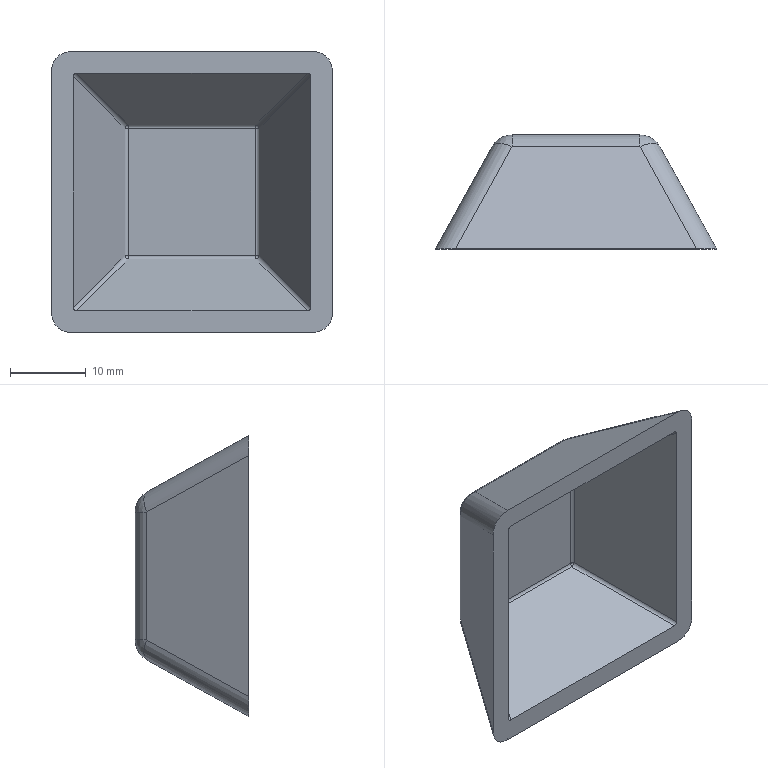Part | SolidWorks | features Extrusion 1, Fillet 1, Shell 1 | 1 solid | 35 faces | box 37 x 15 x 37 mm | volume 4957 mm3 | cylinder 16 | plane 11 | sphere 8 | commonest cylinder face diameters 1 x8 6 x8
STEP:
#1=CARTESIAN_POINT('',(-11.042,13.454,8.418));
#2=VERTEX_POINT('',#1);
#3=CARTESIAN_POINT('',(-11.042,13.454,-8.418));
#4=VERTEX_POINT('',#3);
#5=CARTESIAN_POINT('',(-11.042,13.454,-10.185));
#6=DIRECTION('',(0.,0.,-1.));
#7=VECTOR('',#6,1000.);
#8=LINE('',#5,#7);
#9=EDGE_CURVE('',#2,#4,#8,.T.);
#10=ORIENTED_EDGE('',*,*,#9,.T.);
#11=CARTESIAN_POINT('',(-18.5,0.,-15.876));
#12=VERTEX_POINT('',#11);
#13=CARTESIAN_POINT('',(-11.958,11.802,-9.334));
#14=DIRECTION('',(-0.4362,-0.787,-0.4362));
#15=VECTOR('',#14,1000.);
#16=LINE('',#13,#15);
#17=EDGE_CURVE('',#4,#12,#16,.T.);
#18=ORIENTED_EDGE('',*,*,#17,.T.);
#19=CARTESIAN_POINT('',(-18.5,0.,15.876));
#20=VERTEX_POINT('',#19);
#21=CARTESIAN_POINT('',(-18.5,0.,18.5));
#22=DIRECTION('',(0.,0.,-1.));
#23=VECTOR('',#22,1000.);
#24=LINE('',#21,#23);
#25=EDGE_CURVE('',#20,#12,#24,.T.);
#26=ORIENTED_EDGE('',*,*,#25,.F.);
#27=CARTESIAN_POINT('',(-10.685,14.099,8.061));
#28=DIRECTION('',(0.4362,0.787,-0.4362));
#29=VECTOR('',#28,1000.);
#30=LINE('',#27,#29);
#31=EDGE_CURVE('',#20,#2,#30,.T.);
#32=ORIENTED_EDGE('',*,*,#31,.T.);
#33=EDGE_LOOP('',(#10,#18,#26,#32));
#34=FACE_OUTER_BOUND('',#33,.T.);
#35=CARTESIAN_POINT('',(-18.5,0.,18.5));
#36=DIRECTION('',(-0.8746,0.4848,0.));
#37=DIRECTION('',(-0.4848,-0.8746,0.));
#38=AXIS2_PLACEMENT_3D('',#35,#36,#37);
#39=PLANE('',#38);
#40=ADVANCED_FACE('',(#34),#39,.T.);
#41=CARTESIAN_POINT('',(-15.876,0.,18.5));
#42=VERTEX_POINT('',#41);
#43=CARTESIAN_POINT('',(15.876,0.,18.5));
#44=VERTEX_POINT('',#43);
#45=CARTESIAN_POINT('',(-18.5,0.,18.5));
#46=DIRECTION('',(1.,0.,0.));
#47=VECTOR('',#46,1000.);
#48=LINE('',#45,#47);
#49=EDGE_CURVE('',#42,#44,#48,.T.);
#50=ORIENTED_EDGE('',*,*,#49,.T.);
#51=CARTESIAN_POINT('',(8.418,13.454,11.042));
#52=VERTEX_POINT('',#51);
#53=CARTESIAN_POINT('',(9.334,11.802,11.958));
#54=DIRECTION('',(-0.4362,0.787,-0.4362));
#55=VECTOR('',#54,1000.);
#56=LINE('',#53,#55);
#57=EDGE_CURVE('',#44,#52,#56,.T.);
#58=ORIENTED_EDGE('',*,*,#57,.T.);
#59=CARTESIAN_POINT('',(-8.418,13.454,11.042));
#60=VERTEX_POINT('',#59);
#61=CARTESIAN_POINT('',(-18.5,13.454,11.042));
#62=DIRECTION('',(-1.,0.,0.));
#63=VECTOR('',#62,1000.);
#64=LINE('',#61,#63);
#65=EDGE_CURVE('',#52,#60,#64,.T.);
#66=ORIENTED_EDGE('',*,*,#65,.T.);
#67=CARTESIAN_POINT('',(-16.375,-0.9008,18.999));
#68=DIRECTION('',(-0.4362,-0.787,0.4362));
#69=VECTOR('',#68,1000.);
#70=LINE('',#67,#69);
#71=EDGE_CURVE('',#60,#42,#70,.T.);
#72=ORIENTED_EDGE('',*,*,#71,.T.);
#73=EDGE_LOOP('',(#50,#58,#66,#72));
#74=FACE_OUTER_BOUND('',#73,.T.);
#75=CARTESIAN_POINT('',(-18.5,0.,18.5));
#76=DIRECTION('',(0.,0.4848,0.8746));
#77=DIRECTION('',(0.,-0.8746,0.4848));
#78=AXIS2_PLACEMENT_3D('',#75,#76,#77);
#79=PLANE('',#78);
#80=ADVANCED_FACE('',(#74),#79,.T.);
#81=CARTESIAN_POINT('',(18.5,0.,15.876));
#82=VERTEX_POINT('',#81);
#83=CARTESIAN_POINT('',(18.5,0.,-15.876));
#84=VERTEX_POINT('',#83);
#85=CARTESIAN_POINT('',(18.5,0.,18.5));
#86=DIRECTION('',(0.,0.,-1.));
#87=VECTOR('',#86,1000.);
#88=LINE('',#85,#87);
#89=EDGE_CURVE('',#82,#84,#88,.T.);
#90=ORIENTED_EDGE('',*,*,#89,.T.);
#91=CARTESIAN_POINT('',(11.042,13.454,-8.418));
#92=VERTEX_POINT('',#91);
#93=CARTESIAN_POINT('',(10.685,14.099,-8.061));
#94=DIRECTION('',(-0.4362,0.787,0.4362));
#95=VECTOR('',#94,1000.);
#96=LINE('',#93,#95);
#97=EDGE_CURVE('',#84,#92,#96,.T.);
#98=ORIENTED_EDGE('',*,*,#97,.T.);
#99=CARTESIAN_POINT('',(11.042,13.454,8.418));
#100=VERTEX_POINT('',#99);
#101=CARTESIAN_POINT('',(11.042,13.454,18.5));
#102=DIRECTION('',(0.,0.,1.));
#103=VECTOR('',#102,1000.);
#104=LINE('',#101,#103);
#105=EDGE_CURVE('',#92,#100,#104,.T.);
#106=ORIENTED_EDGE('',*,*,#105,.T.);
#107=CARTESIAN_POINT('',(18.999,-0.9008,16.375));
#108=DIRECTION('',(0.4362,-0.787,0.4362));
#109=VECTOR('',#108,1000.);
#110=LINE('',#107,#109);
#111=EDGE_CURVE('',#100,#82,#110,.T.);
#112=ORIENTED_EDGE('',*,*,#111,.T.);
#113=EDGE_LOOP('',(#90,#98,#106,#112));
#114=FACE_OUTER_BOUND('',#113,.T.);
#115=CARTESIAN_POINT('',(18.5,0.,18.5));
#116=DIRECTION('',(0.8746,0.4848,0.));
#117=DIRECTION('',(-0.4848,0.8746,0.));
#118=AXIS2_PLACEMENT_3D('',#115,#116,#117);
#119=PLANE('',#118);
#120=ADVANCED_FACE('',(#114),#119,.T.);
#121=CARTESIAN_POINT('',(-8.418,13.454,-11.042));
#122=VERTEX_POINT('',#121);
#123=CARTESIAN_POINT('',(8.418,13.454,-11.042));
#124=VERTEX_POINT('',#123);
#125=CARTESIAN_POINT('',(10.185,13.454,-11.042));
#126=DIRECTION('',(1.,0.,0.));
#127=VECTOR('',#126,1000.);
#128=LINE('',#125,#127);
#129=EDGE_CURVE('',#122,#124,#128,.T.);
#130=ORIENTED_EDGE('',*,*,#129,.T.);
#131=CARTESIAN_POINT('',(15.876,0.,-18.5));
#132=VERTEX_POINT('',#131);
#133=CARTESIAN_POINT('',(16.375,-0.9008,-18.999));
#134=DIRECTION('',(0.4362,-0.787,-0.4362));
#135=VECTOR('',#134,1000.);
#136=LINE('',#133,#135);
#137=EDGE_CURVE('',#124,#132,#136,.T.);
#138=ORIENTED_EDGE('',*,*,#137,.T.);
#139=CARTESIAN_POINT('',(-15.876,0.,-18.5));
#140=VERTEX_POINT('',#139);
#141=CARTESIAN_POINT('',(-18.5,0.,-18.5));
#142=DIRECTION('',(1.,0.,0.));
#143=VECTOR('',#142,1000.);
#144=LINE('',#141,#143);
#145=EDGE_CURVE('',#140,#132,#144,.T.);
#146=ORIENTED_EDGE('',*,*,#145,.F.);
#147=CARTESIAN_POINT('',(-16.375,-0.9008,-18.999));
#148=DIRECTION('',(0.4362,0.787,0.4362));
#149=VECTOR('',#148,1000.);
#150=LINE('',#147,#149);
#151=EDGE_CURVE('',#140,#122,#150,.T.);
#152=ORIENTED_EDGE('',*,*,#151,.T.);
#153=EDGE_LOOP('',(#130,#138,#146,#152));
#154=FACE_OUTER_BOUND('',#153,.T.);
#155=CARTESIAN_POINT('',(-18.5,0.,-18.5));
#156=DIRECTION('',(0.,0.4848,-0.8746));
#157=DIRECTION('',(0.,0.8746,0.4848));
#158=AXIS2_PLACEMENT_3D('',#155,#156,#157);
#159=PLANE('',#158);
#160=ADVANCED_FACE('',(#154),#159,.T.);
#161=CARTESIAN_POINT('',(8.418,15.,8.418));
#162=VERTEX_POINT('',#161);
#163=CARTESIAN_POINT('',(8.418,15.,-8.418));
#164=VERTEX_POINT('',#163);
#165=CARTESIAN_POINT('',(8.418,15.,0.));
#166=DIRECTION('',(0.,0.,-1.));
#167=VECTOR('',#166,1000.);
#168=LINE('',#165,#167);
#169=EDGE_CURVE('',#162,#164,#168,.T.);
#170=ORIENTED_EDGE('',*,*,#169,.T.);
#171=CARTESIAN_POINT('',(-8.418,15.,-8.418));
#172=VERTEX_POINT('',#171);
#173=CARTESIAN_POINT('',(-10.185,15.,-8.418));
#174=DIRECTION('',(-1.,0.,0.));
#175=VECTOR('',#174,1000.);
#176=LINE('',#173,#175);
#177=EDGE_CURVE('',#164,#172,#176,.T.);
#178=ORIENTED_EDGE('',*,*,#177,.T.);
#179=CARTESIAN_POINT('',(-8.418,15.,8.418));
#180=VERTEX_POINT('',#179);
#181=CARTESIAN_POINT('',(-8.418,15.,10.185));
#182=DIRECTION('',(0.,0.,1.));
#183=VECTOR('',#182,1000.);
#184=LINE('',#181,#183);
#185=EDGE_CURVE('',#172,#180,#184,.T.);
#186=ORIENTED_EDGE('',*,*,#185,.T.);
#187=CARTESIAN_POINT('',(0.,15.,8.418));
#188=DIRECTION('',(1.,0.,0.));
#189=VECTOR('',#188,1000.);
#190=LINE('',#187,#189);
#191=EDGE_CURVE('',#180,#162,#190,.T.);
#192=ORIENTED_EDGE('',*,*,#191,.T.);
#193=EDGE_LOOP('',(#170,#178,#186,#192));
#194=FACE_OUTER_BOUND('',#193,.T.);
#195=CARTESIAN_POINT('',(0.,15.,0.));
#196=DIRECTION('',(0.,-1.,0.));
#197=DIRECTION('',(0.,0.,-1.));
#198=AXIS2_PLACEMENT_3D('',#195,#196,#197);
#199=PLANE('',#198);
#200=ADVANCED_FACE('',(#194),#199,.F.);
#201=CARTESIAN_POINT('',(-15.204,0.,-15.642));
#202=VERTEX_POINT('',#201);
#203=CARTESIAN_POINT('',(15.204,0.,-15.642));
#204=VERTEX_POINT('',#203);
#205=CARTESIAN_POINT('',(0.,0.,-15.642));
#206=DIRECTION('',(1.,0.,0.));
#207=VECTOR('',#206,1000.);
#208=LINE('',#205,#207);
#209=EDGE_CURVE('',#202,#204,#208,.T.);
#210=ORIENTED_EDGE('',*,*,#209,.F.);
#211=CARTESIAN_POINT('',(-15.642,0.,-15.204));
#212=VERTEX_POINT('',#211);
#213=CARTESIAN_POINT('',(-15.642,0.,-15.204));
#214=CARTESIAN_POINT('',(-15.642,0.,-15.472));
#215=CARTESIAN_POINT('',(-15.472,0.,-15.642));
#216=CARTESIAN_POINT('',(-15.204,0.,-15.642));
#217=(BOUNDED_CURVE()B_SPLINE_CURVE(3,(#213,#214,#215,#216),.UNSPECIFIED.,.F.,.T.)B_SPLINE_CURVE_WITH_KNOTS((4,4),(5.616,6.95),.UNSPECIFIED.)CURVE()GEOMETRIC_REPRESENTATION_ITEM()RATIONAL_B_SPLINE_CURVE((1.,0.8572,0.8572,1.))REPRESENTATION_ITEM(''));
#218=EDGE_CURVE('',#212,#202,#217,.T.);
#219=ORIENTED_EDGE('',*,*,#218,.F.);
#220=CARTESIAN_POINT('',(-15.642,0.,15.204));
#221=VERTEX_POINT('',#220);
#222=CARTESIAN_POINT('',(-15.642,0.,0.));
#223=DIRECTION('',(0.,0.,-1.));
#224=VECTOR('',#223,1000.);
#225=LINE('',#222,#224);
#226=EDGE_CURVE('',#221,#212,#225,.T.);
#227=ORIENTED_EDGE('',*,*,#226,.F.);
#228=CARTESIAN_POINT('',(-15.204,0.,15.642));
#229=VERTEX_POINT('',#228);
#230=CARTESIAN_POINT('',(-15.204,0.,15.642));
#231=CARTESIAN_POINT('',(-15.472,0.,15.642));
#232=CARTESIAN_POINT('',(-15.642,0.,15.472));
#233=CARTESIAN_POINT('',(-15.642,0.,15.204));
#234=(BOUNDED_CURVE()B_SPLINE_CURVE(3,(#230,#231,#232,#233),.UNSPECIFIED.,.F.,.T.)B_SPLINE_CURVE_WITH_KNOTS((4,4),(5.616,6.95),.UNSPECIFIED.)CURVE()GEOMETRIC_REPRESENTATION_ITEM()RATIONAL_B_SPLINE_CURVE((1.,0.8572,0.8572,1.))REPRESENTATION_ITEM(''));
#235=EDGE_CURVE('',#229,#221,#234,.T.);
#236=ORIENTED_EDGE('',*,*,#235,.F.);
#237=CARTESIAN_POINT('',(15.204,0.,15.642));
#238=VERTEX_POINT('',#237);
#239=CARTESIAN_POINT('',(0.,0.,15.642));
#240=DIRECTION('',(1.,0.,0.));
#241=VECTOR('',#240,1000.);
#242=LINE('',#239,#241);
#243=EDGE_CURVE('',#229,#238,#242,.T.);
#244=ORIENTED_EDGE('',*,*,#243,.T.);
#245=CARTESIAN_POINT('',(15.642,0.,15.204));
#246=VERTEX_POINT('',#245);
#247=CARTESIAN_POINT('',(15.642,0.,15.204));
#248=CARTESIAN_POINT('',(15.642,0.,15.472));
#249=CARTESIAN_POINT('',(15.472,0.,15.642));
#250=CARTESIAN_POINT('',(15.204,0.,15.642));
#251=(BOUNDED_CURVE()B_SPLINE_CURVE(3,(#247,#248,#249,#250),.UNSPECIFIED.,.F.,.T.)B_SPLINE_CURVE_WITH_KNOTS((4,4),(5.616,6.95),.UNSPECIFIED.)CURVE()GEOMETRIC_REPRESENTATION_ITEM()RATIONAL_B_SPLINE_CURVE((1.,0.8572,0.8572,1.))REPRESENTATION_ITEM(''));
#252=EDGE_CURVE('',#246,#238,#251,.T.);
#253=ORIENTED_EDGE('',*,*,#252,.F.);
#254=CARTESIAN_POINT('',(15.642,0.,-15.204));
#255=VERTEX_POINT('',#254);
#256=CARTESIAN_POINT('',(15.642,0.,0.));
#257=DIRECTION('',(0.,0.,-1.));
#258=VECTOR('',#257,1000.);
#259=LINE('',#256,#258);
#260=EDGE_CURVE('',#246,#255,#259,.T.);
#261=ORIENTED_EDGE('',*,*,#260,.T.);
#262=CARTESIAN_POINT('',(15.204,0.,-15.642));
#263=CARTESIAN_POINT('',(15.472,0.,-15.642));
#264=CARTESIAN_POINT('',(15.642,0.,-15.472));
#265=CARTESIAN_POINT('',(15.642,0.,-15.204));
#266=(BOUNDED_CURVE()B_SPLINE_CURVE(3,(#262,#263,#264,#265),.UNSPECIFIED.,.F.,.T.)B_SPLINE_CURVE_WITH_KNOTS((4,4),(5.616,6.95),.UNSPECIFIED.)CURVE()GEOMETRIC_REPRESENTATION_ITEM()RATIONAL_B_SPLINE_CURVE((1.,0.8572,0.8572,1.))REPRESENTATION_ITEM(''));
#267=EDGE_CURVE('',#204,#255,#266,.T.);
#268=ORIENTED_EDGE('',*,*,#267,.F.);
#269=EDGE_LOOP('',(#210,#219,#227,#236,#244,#253,#261,#268));
#270=FACE_BOUND('',#269,.T.);
#271=ORIENTED_EDGE('',*,*,#145,.T.);
#272=CARTESIAN_POINT('',(15.876,0.,-18.5));
#273=CARTESIAN_POINT('',(17.48,0.,-18.5));
#274=CARTESIAN_POINT('',(18.5,0.,-17.48));
#275=CARTESIAN_POINT('',(18.5,0.,-15.876));
#276=(BOUNDED_CURVE()B_SPLINE_CURVE(3,(#272,#273,#274,#275),.UNSPECIFIED.,.F.,.T.)B_SPLINE_CURVE_WITH_KNOTS((4,4),(5.616,6.95),.UNSPECIFIED.)CURVE()GEOMETRIC_REPRESENTATION_ITEM()RATIONAL_B_SPLINE_CURVE((1.,0.8572,0.8572,1.))REPRESENTATION_ITEM(''));
#277=EDGE_CURVE('',#132,#84,#276,.T.);
#278=ORIENTED_EDGE('',*,*,#277,.T.);
#279=ORIENTED_EDGE('',*,*,#89,.F.);
#280=CARTESIAN_POINT('',(18.5,0.,15.876));
#281=CARTESIAN_POINT('',(18.5,0.,17.48));
#282=CARTESIAN_POINT('',(17.48,0.,18.5));
#283=CARTESIAN_POINT('',(15.876,0.,18.5));
#284=(BOUNDED_CURVE()B_SPLINE_CURVE(3,(#280,#281,#282,#283),.UNSPECIFIED.,.F.,.T.)B_SPLINE_CURVE_WITH_KNOTS((4,4),(5.616,6.95),.UNSPECIFIED.)CURVE()GEOMETRIC_REPRESENTATION_ITEM()RATIONAL_B_SPLINE_CURVE((1.,0.8572,0.8572,1.))REPRESENTATION_ITEM(''));
#285=EDGE_CURVE('',#82,#44,#284,.T.);
#286=ORIENTED_EDGE('',*,*,#285,.T.);
#287=ORIENTED_EDGE('',*,*,#49,.F.);
#288=CARTESIAN_POINT('',(-15.876,0.,18.5));
#289=CARTESIAN_POINT('',(-17.48,0.,18.5));
#290=CARTESIAN_POINT('',(-18.5,0.,17.48));
#291=CARTESIAN_POINT('',(-18.5,0.,15.876));
#292=(BOUNDED_CURVE()B_SPLINE_CURVE(3,(#288,#289,#290,#291),.UNSPECIFIED.,.F.,.T.)B_SPLINE_CURVE_WITH_KNOTS((4,4),(5.616,6.95),.UNSPECIFIED.)CURVE()GEOMETRIC_REPRESENTATION_ITEM()RATIONAL_B_SPLINE_CURVE((1.,0.8572,0.8572,1.))REPRESENTATION_ITEM(''));
#293=EDGE_CURVE('',#42,#20,#292,.T.);
#294=ORIENTED_EDGE('',*,*,#293,.T.);
#295=ORIENTED_EDGE('',*,*,#25,.T.);
#296=CARTESIAN_POINT('',(-18.5,0.,-15.876));
#297=CARTESIAN_POINT('',(-18.5,0.,-17.48));
#298=CARTESIAN_POINT('',(-17.48,0.,-18.5));
#299=CARTESIAN_POINT('',(-15.876,0.,-18.5));
#300=(BOUNDED_CURVE()B_SPLINE_CURVE(3,(#296,#297,#298,#299),.UNSPECIFIED.,.F.,.T.)B_SPLINE_CURVE_WITH_KNOTS((4,4),(5.616,6.95),.UNSPECIFIED.)CURVE()GEOMETRIC_REPRESENTATION_ITEM()RATIONAL_B_SPLINE_CURVE((1.,0.8572,0.8572,1.))REPRESENTATION_ITEM(''));
#301=EDGE_CURVE('',#12,#140,#300,.T.);
#302=ORIENTED_EDGE('',*,*,#301,.T.);
#303=EDGE_LOOP('',(#271,#278,#279,#286,#287,#294,#295,#302));
#304=FACE_OUTER_BOUND('',#303,.T.);
#305=CARTESIAN_POINT('',(0.,0.,0.));
#306=DIRECTION('',(0.,-1.,0.));
#307=DIRECTION('',(0.,0.,-1.));
#308=AXIS2_PLACEMENT_3D('',#305,#306,#307);
#309=PLANE('',#308);
#310=ADVANCED_FACE('',(#270,#304),#309,.T.);
#311=ORIENTED_EDGE('',*,*,#293,.F.);
#312=ORIENTED_EDGE('',*,*,#71,.F.);
#313=CARTESIAN_POINT('',(-8.418,12.,8.418));
#314=DIRECTION('',(0.4362,0.787,-0.4362));
#315=DIRECTION('',(0.,0.4848,0.8746));
#316=AXIS2_PLACEMENT_3D('',#313,#314,#315);
#317=CIRCLE('',#316,3.);
#318=EDGE_CURVE('',#2,#60,#317,.T.);
#319=ORIENTED_EDGE('',*,*,#318,.F.);
#320=ORIENTED_EDGE('',*,*,#31,.F.);
#321=EDGE_LOOP('',(#311,#312,#319,#320));
#322=FACE_OUTER_BOUND('',#321,.T.);
#323=CARTESIAN_POINT('',(-16.375,-2.355,16.375));
#324=DIRECTION('',(-0.4362,-0.787,0.4362));
#325=DIRECTION('',(0.,-0.4848,-0.8746));
#326=AXIS2_PLACEMENT_3D('',#323,#324,#325);
#327=CYLINDRICAL_SURFACE('',#326,3.);
#328=ADVANCED_FACE('',(#322),#327,.T.);
#329=ORIENTED_EDGE('',*,*,#285,.F.);
#330=ORIENTED_EDGE('',*,*,#111,.F.);
#331=CARTESIAN_POINT('',(8.418,12.,8.418));
#332=DIRECTION('',(-0.4362,0.787,-0.4362));
#333=DIRECTION('',(-0.8746,-0.4848,0.));
#334=AXIS2_PLACEMENT_3D('',#331,#332,#333);
#335=CIRCLE('',#334,3.);
#336=EDGE_CURVE('',#52,#100,#335,.T.);
#337=ORIENTED_EDGE('',*,*,#336,.F.);
#338=ORIENTED_EDGE('',*,*,#57,.F.);
#339=EDGE_LOOP('',(#329,#330,#337,#338));
#340=FACE_OUTER_BOUND('',#339,.T.);
#341=CARTESIAN_POINT('',(16.375,-2.355,16.375));
#342=DIRECTION('',(0.4362,-0.787,0.4362));
#343=DIRECTION('',(0.,-0.4848,-0.8746));
#344=AXIS2_PLACEMENT_3D('',#341,#342,#343);
#345=CYLINDRICAL_SURFACE('',#344,3.);
#346=ADVANCED_FACE('',(#340),#345,.T.);
#347=CARTESIAN_POINT('',(-8.418,12.,8.418));
#348=DIRECTION('',(-1.,0.,0.));
#349=DIRECTION('',(0.,0.,1.));
#350=AXIS2_PLACEMENT_3D('',#347,#348,#349);
#351=CIRCLE('',#350,3.);
#352=EDGE_CURVE('',#60,#180,#351,.T.);
#353=ORIENTED_EDGE('',*,*,#352,.F.);
#354=ORIENTED_EDGE('',*,*,#65,.F.);
#355=CARTESIAN_POINT('',(8.418,12.,8.418));
#356=DIRECTION('',(1.,0.,0.));
#357=DIRECTION('',(0.,0.,-1.));
#358=AXIS2_PLACEMENT_3D('',#355,#356,#357);
#359=CIRCLE('',#358,3.);
#360=EDGE_CURVE('',#162,#52,#359,.T.);
#361=ORIENTED_EDGE('',*,*,#360,.F.);
#362=ORIENTED_EDGE('',*,*,#191,.F.);
#363=EDGE_LOOP('',(#353,#354,#361,#362));
#364=FACE_OUTER_BOUND('',#363,.T.);
#365=CARTESIAN_POINT('',(0.,12.,8.418));
#366=DIRECTION('',(-1.,0.,0.));
#367=DIRECTION('',(0.,0.,1.));
#368=AXIS2_PLACEMENT_3D('',#365,#366,#367);
#369=CYLINDRICAL_SURFACE('',#368,3.);
#370=ADVANCED_FACE('',(#364),#369,.T.);
#371=ORIENTED_EDGE('',*,*,#318,.T.);
#372=ORIENTED_EDGE('',*,*,#352,.T.);
#373=CARTESIAN_POINT('',(-8.418,12.,8.418));
#374=DIRECTION('',(0.,0.,-1.));
#375=DIRECTION('',(1.,0.,0.));
#376=AXIS2_PLACEMENT_3D('',#373,#374,#375);
#377=CIRCLE('',#376,3.);
#378=EDGE_CURVE('',#2,#180,#377,.T.);
#379=ORIENTED_EDGE('',*,*,#378,.F.);
#380=EDGE_LOOP('',(#371,#372,#379));
#381=FACE_OUTER_BOUND('',#380,.T.);
#382=CARTESIAN_POINT('',(-8.418,12.,8.418));
#383=DIRECTION('',(1.,0.,0.));
#384=DIRECTION('',(0.,0.,1.));
#385=AXIS2_PLACEMENT_3D('',#382,#383,#384);
#386=SPHERICAL_SURFACE('',#385,3.);
#387=ADVANCED_FACE('',(#381),#386,.T.);
#388=ORIENTED_EDGE('',*,*,#360,.T.);
#389=ORIENTED_EDGE('',*,*,#336,.T.);
#390=CARTESIAN_POINT('',(8.418,12.,8.418));
#391=DIRECTION('',(0.,0.,-1.));
#392=DIRECTION('',(1.,0.,0.));
#393=AXIS2_PLACEMENT_3D('',#390,#391,#392);
#394=CIRCLE('',#393,3.);
#395=EDGE_CURVE('',#162,#100,#394,.T.);
#396=ORIENTED_EDGE('',*,*,#395,.F.);
#397=EDGE_LOOP('',(#388,#389,#396));
#398=FACE_OUTER_BOUND('',#397,.T.);
#399=CARTESIAN_POINT('',(8.418,12.,8.418));
#400=DIRECTION('',(1.,0.,0.));
#401=DIRECTION('',(0.,0.,1.));
#402=AXIS2_PLACEMENT_3D('',#399,#400,#401);
#403=SPHERICAL_SURFACE('',#402,3.);
#404=ADVANCED_FACE('',(#398),#403,.T.);
#405=ORIENTED_EDGE('',*,*,#378,.T.);
#406=ORIENTED_EDGE('',*,*,#185,.F.);
#407=CARTESIAN_POINT('',(-8.418,12.,-8.418));
#408=DIRECTION('',(0.,0.,-1.));
#409=DIRECTION('',(-1.,0.,0.));
#410=AXIS2_PLACEMENT_3D('',#407,#408,#409);
#411=CIRCLE('',#410,3.);
#412=EDGE_CURVE('',#4,#172,#411,.T.);
#413=ORIENTED_EDGE('',*,*,#412,.F.);
#414=ORIENTED_EDGE('',*,*,#9,.F.);
#415=EDGE_LOOP('',(#405,#406,#413,#414));
#416=FACE_OUTER_BOUND('',#415,.T.);
#417=CARTESIAN_POINT('',(-8.418,12.,18.5));
#418=DIRECTION('',(0.,0.,1.));
#419=DIRECTION('',(1.,0.,0.));
#420=AXIS2_PLACEMENT_3D('',#417,#418,#419);
#421=CYLINDRICAL_SURFACE('',#420,3.);
#422=ADVANCED_FACE('',(#416),#421,.T.);
#423=ORIENTED_EDGE('',*,*,#301,.F.);
#424=ORIENTED_EDGE('',*,*,#17,.F.);
#425=CARTESIAN_POINT('',(-8.418,12.,-8.418));
#426=DIRECTION('',(0.4362,0.787,0.4362));
#427=DIRECTION('',(0.,-0.4848,0.8746));
#428=AXIS2_PLACEMENT_3D('',#425,#426,#427);
#429=CIRCLE('',#428,3.);
#430=EDGE_CURVE('',#122,#4,#429,.T.);
#431=ORIENTED_EDGE('',*,*,#430,.F.);
#432=ORIENTED_EDGE('',*,*,#151,.F.);
#433=EDGE_LOOP('',(#423,#424,#431,#432));
#434=FACE_OUTER_BOUND('',#433,.T.);
#435=CARTESIAN_POINT('',(-9.334,10.348,-9.334));
#436=DIRECTION('',(-0.4362,-0.787,-0.4362));
#437=DIRECTION('',(0.,0.4848,-0.8746));
#438=AXIS2_PLACEMENT_3D('',#435,#436,#437);
#439=CYLINDRICAL_SURFACE('',#438,3.);
#440=ADVANCED_FACE('',(#434),#439,.T.);
#441=ORIENTED_EDGE('',*,*,#277,.F.);
#442=ORIENTED_EDGE('',*,*,#137,.F.);
#443=CARTESIAN_POINT('',(8.418,12.,-8.418));
#444=DIRECTION('',(-0.4362,0.787,0.4362));
#445=DIRECTION('',(-0.8746,-0.4848,0.));
#446=AXIS2_PLACEMENT_3D('',#443,#444,#445);
#447=CIRCLE('',#446,3.);
#448=EDGE_CURVE('',#92,#124,#447,.T.);
#449=ORIENTED_EDGE('',*,*,#448,.F.);
#450=ORIENTED_EDGE('',*,*,#97,.F.);
#451=EDGE_LOOP('',(#441,#442,#449,#450));
#452=FACE_OUTER_BOUND('',#451,.T.);
#453=CARTESIAN_POINT('',(9.334,10.348,-9.334));
#454=DIRECTION('',(0.4362,-0.787,-0.4362));
#455=DIRECTION('',(0.,0.4848,-0.8746));
#456=AXIS2_PLACEMENT_3D('',#453,#454,#455);
#457=CYLINDRICAL_SURFACE('',#456,3.);
#458=ADVANCED_FACE('',(#452),#457,.T.);
#459=ORIENTED_EDGE('',*,*,#395,.T.);
#460=ORIENTED_EDGE('',*,*,#105,.F.);
#461=CARTESIAN_POINT('',(8.418,12.,-8.418));
#462=DIRECTION('',(0.,0.,-1.));
#463=DIRECTION('',(-1.,0.,0.));
#464=AXIS2_PLACEMENT_3D('',#461,#462,#463);
#465=CIRCLE('',#464,3.);
#466=EDGE_CURVE('',#164,#92,#465,.T.);
#467=ORIENTED_EDGE('',*,*,#466,.F.);
#468=ORIENTED_EDGE('',*,*,#169,.F.);
#469=EDGE_LOOP('',(#459,#460,#467,#468));
#470=FACE_OUTER_BOUND('',#469,.T.);
#471=CARTESIAN_POINT('',(8.418,12.,0.));
#472=DIRECTION('',(0.,0.,1.));
#473=DIRECTION('',(1.,0.,0.));
#474=AXIS2_PLACEMENT_3D('',#471,#472,#473);
#475=CYLINDRICAL_SURFACE('',#474,3.);
#476=ADVANCED_FACE('',(#470),#475,.T.);
#477=ORIENTED_EDGE('',*,*,#430,.T.);
#478=ORIENTED_EDGE('',*,*,#412,.T.);
#479=CARTESIAN_POINT('',(-8.418,12.,-8.418));
#480=DIRECTION('',(1.,0.,0.));
#481=DIRECTION('',(0.,0.,1.));
#482=AXIS2_PLACEMENT_3D('',#479,#480,#481);
#483=CIRCLE('',#482,3.);
#484=EDGE_CURVE('',#122,#172,#483,.T.);
#485=ORIENTED_EDGE('',*,*,#484,.F.);
#486=EDGE_LOOP('',(#477,#478,#485));
#487=FACE_OUTER_BOUND('',#486,.T.);
#488=CARTESIAN_POINT('',(-8.418,12.,-8.418));
#489=DIRECTION('',(0.,0.,1.));
#490=DIRECTION('',(-1.,0.,0.));
#491=AXIS2_PLACEMENT_3D('',#488,#489,#490);
#492=SPHERICAL_SURFACE('',#491,3.);
#493=ADVANCED_FACE('',(#487),#492,.T.);
#494=ORIENTED_EDGE('',*,*,#466,.T.);
#495=ORIENTED_EDGE('',*,*,#448,.T.);
#496=CARTESIAN_POINT('',(8.418,12.,-8.418));
#497=DIRECTION('',(-1.,0.,0.));
#498=DIRECTION('',(0.,1.,0.));
#499=AXIS2_PLACEMENT_3D('',#496,#497,#498);
#500=CIRCLE('',#499,3.);
#501=EDGE_CURVE('',#164,#124,#500,.T.);
#502=ORIENTED_EDGE('',*,*,#501,.F.);
#503=EDGE_LOOP('',(#494,#495,#502));
#504=FACE_OUTER_BOUND('',#503,.T.);
#505=CARTESIAN_POINT('',(8.418,12.,-8.418));
#506=DIRECTION('',(1.,0.,0.));
#507=DIRECTION('',(0.,0.,1.));
#508=AXIS2_PLACEMENT_3D('',#505,#506,#507);
#509=SPHERICAL_SURFACE('',#508,3.);
#510=ADVANCED_FACE('',(#504),#509,.T.);
#511=ORIENTED_EDGE('',*,*,#484,.T.);
#512=ORIENTED_EDGE('',*,*,#177,.F.);
#513=ORIENTED_EDGE('',*,*,#501,.T.);
#514=ORIENTED_EDGE('',*,*,#129,.F.);
#515=EDGE_LOOP('',(#511,#512,#513,#514));
#516=FACE_OUTER_BOUND('',#515,.T.);
#517=CARTESIAN_POINT('',(-18.5,12.,-8.418));
#518=DIRECTION('',(-1.,0.,0.));
#519=DIRECTION('',(0.,0.,1.));
#520=AXIS2_PLACEMENT_3D('',#517,#518,#519);
#521=CYLINDRICAL_SURFACE('',#520,3.);
#522=ADVANCED_FACE('',(#516),#521,.T.);
#523=CARTESIAN_POINT('',(-8.856,12.242,8.418));
#524=VERTEX_POINT('',#523);
#525=CARTESIAN_POINT('',(-8.856,12.242,-8.418));
#526=VERTEX_POINT('',#525);
#527=CARTESIAN_POINT('',(-8.856,12.242,18.5));
#528=DIRECTION('',(0.,0.,-1.));
#529=VECTOR('',#528,1000.);
#530=LINE('',#527,#529);
#531=EDGE_CURVE('',#524,#526,#530,.T.);
#532=ORIENTED_EDGE('',*,*,#531,.F.);
#533=CARTESIAN_POINT('',(-16.813,-2.113,16.375));
#534=DIRECTION('',(0.4362,0.787,-0.4362));
#535=VECTOR('',#534,1000.);
#536=LINE('',#533,#535);
#537=EDGE_CURVE('',#221,#524,#536,.T.);
#538=ORIENTED_EDGE('',*,*,#537,.F.);
#539=ORIENTED_EDGE('',*,*,#226,.T.);
#540=CARTESIAN_POINT('',(-9.771,10.59,-9.334));
#541=DIRECTION('',(-0.4362,-0.787,-0.4362));
#542=VECTOR('',#541,1000.);
#543=LINE('',#540,#542);
#544=EDGE_CURVE('',#526,#212,#543,.T.);
#545=ORIENTED_EDGE('',*,*,#544,.F.);
#546=EDGE_LOOP('',(#532,#538,#539,#545));
#547=FACE_OUTER_BOUND('',#546,.T.);
#548=CARTESIAN_POINT('',(-16.313,-1.212,18.5));
#549=DIRECTION('',(-0.8746,0.4848,0.));
#550=DIRECTION('',(-0.4848,-0.8746,0.));
#551=AXIS2_PLACEMENT_3D('',#548,#549,#550);
#552=PLANE('',#551);
#553=ADVANCED_FACE('',(#547),#552,.F.);
#554=ORIENTED_EDGE('',*,*,#243,.F.);
#555=CARTESIAN_POINT('',(-8.418,12.242,8.856));
#556=VERTEX_POINT('',#555);
#557=CARTESIAN_POINT('',(-16.375,-2.113,16.813));
#558=DIRECTION('',(-0.4362,-0.787,0.4362));
#559=VECTOR('',#558,1000.);
#560=LINE('',#557,#559);
#561=EDGE_CURVE('',#556,#229,#560,.T.);
#562=ORIENTED_EDGE('',*,*,#561,.F.);
#563=CARTESIAN_POINT('',(8.418,12.242,8.856));
#564=VERTEX_POINT('',#563);
#565=CARTESIAN_POINT('',(-18.5,12.242,8.856));
#566=DIRECTION('',(-1.,0.,0.));
#567=VECTOR('',#566,1000.);
#568=LINE('',#565,#567);
#569=EDGE_CURVE('',#564,#556,#568,.T.);
#570=ORIENTED_EDGE('',*,*,#569,.F.);
#571=CARTESIAN_POINT('',(16.375,-2.113,16.813));
#572=DIRECTION('',(-0.4362,0.787,-0.4362));
#573=VECTOR('',#572,1000.);
#574=LINE('',#571,#573);
#575=EDGE_CURVE('',#238,#564,#574,.T.);
#576=ORIENTED_EDGE('',*,*,#575,.F.);
#577=EDGE_LOOP('',(#554,#562,#570,#576));
#578=FACE_OUTER_BOUND('',#577,.T.);
#579=CARTESIAN_POINT('',(-18.5,-1.212,16.313));
#580=DIRECTION('',(0.,0.4848,0.8746));
#581=DIRECTION('',(0.,-0.8746,0.4848));
#582=AXIS2_PLACEMENT_3D('',#579,#580,#581);
#583=PLANE('',#582);
#584=ADVANCED_FACE('',(#578),#583,.F.);
#585=ORIENTED_EDGE('',*,*,#260,.F.);
#586=CARTESIAN_POINT('',(8.856,12.242,8.418));
#587=VERTEX_POINT('',#586);
#588=CARTESIAN_POINT('',(16.813,-2.113,16.375));
#589=DIRECTION('',(0.4362,-0.787,0.4362));
#590=VECTOR('',#589,1000.);
#591=LINE('',#588,#590);
#592=EDGE_CURVE('',#587,#246,#591,.T.);
#593=ORIENTED_EDGE('',*,*,#592,.F.);
#594=CARTESIAN_POINT('',(8.856,12.242,-8.418));
#595=VERTEX_POINT('',#594);
#596=CARTESIAN_POINT('',(8.856,12.242,18.5));
#597=DIRECTION('',(0.,0.,1.));
#598=VECTOR('',#597,1000.);
#599=LINE('',#596,#598);
#600=EDGE_CURVE('',#595,#587,#599,.T.);
#601=ORIENTED_EDGE('',*,*,#600,.F.);
#602=CARTESIAN_POINT('',(9.771,10.59,-9.334));
#603=DIRECTION('',(-0.4362,0.787,0.4362));
#604=VECTOR('',#603,1000.);
#605=LINE('',#602,#604);
#606=EDGE_CURVE('',#255,#595,#605,.T.);
#607=ORIENTED_EDGE('',*,*,#606,.F.);
#608=EDGE_LOOP('',(#585,#593,#601,#607));
#609=FACE_OUTER_BOUND('',#608,.T.);
#610=CARTESIAN_POINT('',(16.313,-1.212,18.5));
#611=DIRECTION('',(0.8746,0.4848,0.));
#612=DIRECTION('',(-0.4848,0.8746,0.));
#613=AXIS2_PLACEMENT_3D('',#610,#611,#612);
#614=PLANE('',#613);
#615=ADVANCED_FACE('',(#609),#614,.F.);
#616=CARTESIAN_POINT('',(-8.418,12.242,-8.856));
#617=VERTEX_POINT('',#616);
#618=CARTESIAN_POINT('',(8.418,12.242,-8.856));
#619=VERTEX_POINT('',#618);
#620=CARTESIAN_POINT('',(-18.5,12.242,-8.856));
#621=DIRECTION('',(1.,0.,0.));
#622=VECTOR('',#621,1000.);
#623=LINE('',#620,#622);
#624=EDGE_CURVE('',#617,#619,#623,.T.);
#625=ORIENTED_EDGE('',*,*,#624,.F.);
#626=CARTESIAN_POINT('',(-9.334,10.59,-9.771));
#627=DIRECTION('',(0.4362,0.787,0.4362));
#628=VECTOR('',#627,1000.);
#629=LINE('',#626,#628);
#630=EDGE_CURVE('',#202,#617,#629,.T.);
#631=ORIENTED_EDGE('',*,*,#630,.F.);
#632=ORIENTED_EDGE('',*,*,#209,.T.);
#633=CARTESIAN_POINT('',(9.334,10.59,-9.771));
#634=DIRECTION('',(0.4362,-0.787,-0.4362));
#635=VECTOR('',#634,1000.);
#636=LINE('',#633,#635);
#637=EDGE_CURVE('',#619,#204,#636,.T.);
#638=ORIENTED_EDGE('',*,*,#637,.F.);
#639=EDGE_LOOP('',(#625,#631,#632,#638));
#640=FACE_OUTER_BOUND('',#639,.T.);
#641=CARTESIAN_POINT('',(-18.5,-1.212,-16.313));
#642=DIRECTION('',(0.,0.4848,-0.8746));
#643=DIRECTION('',(0.,0.8746,0.4848));
#644=AXIS2_PLACEMENT_3D('',#641,#642,#643);
#645=PLANE('',#644);
#646=ADVANCED_FACE('',(#640),#645,.F.);
#647=CARTESIAN_POINT('',(8.418,12.5,8.418));
#648=VERTEX_POINT('',#647);
#649=CARTESIAN_POINT('',(8.418,12.5,-8.418));
#650=VERTEX_POINT('',#649);
#651=CARTESIAN_POINT('',(8.418,12.5,0.));
#652=DIRECTION('',(0.,0.,-1.));
#653=VECTOR('',#652,1000.);
#654=LINE('',#651,#653);
#655=EDGE_CURVE('',#648,#650,#654,.T.);
#656=ORIENTED_EDGE('',*,*,#655,.F.);
#657=CARTESIAN_POINT('',(-8.418,12.5,8.418));
#658=VERTEX_POINT('',#657);
#659=CARTESIAN_POINT('',(0.,12.5,8.418));
#660=DIRECTION('',(1.,0.,0.));
#661=VECTOR('',#660,1000.);
#662=LINE('',#659,#661);
#663=EDGE_CURVE('',#658,#648,#662,.T.);
#664=ORIENTED_EDGE('',*,*,#663,.F.);
#665=CARTESIAN_POINT('',(-8.418,12.5,-8.418));
#666=VERTEX_POINT('',#665);
#667=CARTESIAN_POINT('',(-8.418,12.5,0.));
#668=DIRECTION('',(0.,0.,1.));
#669=VECTOR('',#668,1000.);
#670=LINE('',#667,#669);
#671=EDGE_CURVE('',#666,#658,#670,.T.);
#672=ORIENTED_EDGE('',*,*,#671,.F.);
#673=CARTESIAN_POINT('',(0.,12.5,-8.418));
#674=DIRECTION('',(-1.,0.,0.));
#675=VECTOR('',#674,1000.);
#676=LINE('',#673,#675);
#677=EDGE_CURVE('',#650,#666,#676,.T.);
#678=ORIENTED_EDGE('',*,*,#677,.F.);
#679=EDGE_LOOP('',(#656,#664,#672,#678));
#680=FACE_OUTER_BOUND('',#679,.T.);
#681=CARTESIAN_POINT('',(0.,12.5,0.));
#682=DIRECTION('',(0.,-1.,0.));
#683=DIRECTION('',(0.,0.,-1.));
#684=AXIS2_PLACEMENT_3D('',#681,#682,#683);
#685=PLANE('',#684);
#686=ADVANCED_FACE('',(#680),#685,.T.);
#687=ORIENTED_EDGE('',*,*,#235,.T.);
#688=ORIENTED_EDGE('',*,*,#537,.T.);
#689=CARTESIAN_POINT('',(-8.418,12.,8.418));
#690=DIRECTION('',(0.4362,0.787,-0.4362));
#691=DIRECTION('',(0.,-0.4848,-0.8746));
#692=AXIS2_PLACEMENT_3D('',#689,#690,#691);
#693=CIRCLE('',#692,0.5);
#694=EDGE_CURVE('',#524,#556,#693,.T.);
#695=ORIENTED_EDGE('',*,*,#694,.T.);
#696=ORIENTED_EDGE('',*,*,#561,.T.);
#697=EDGE_LOOP('',(#687,#688,#695,#696));
#698=FACE_OUTER_BOUND('',#697,.T.);
#699=CARTESIAN_POINT('',(-16.375,-2.355,16.375));
#700=DIRECTION('',(-0.4362,-0.787,0.4362));
#701=DIRECTION('',(0.,-0.4848,-0.8746));
#702=AXIS2_PLACEMENT_3D('',#699,#700,#701);
#703=CYLINDRICAL_SURFACE('',#702,0.5);
#704=ADVANCED_FACE('',(#698),#703,.F.);
#705=ORIENTED_EDGE('',*,*,#252,.T.);
#706=ORIENTED_EDGE('',*,*,#575,.T.);
#707=CARTESIAN_POINT('',(8.418,12.,8.418));
#708=DIRECTION('',(-0.4362,0.787,-0.4362));
#709=DIRECTION('',(0.,-0.4848,-0.8746));
#710=AXIS2_PLACEMENT_3D('',#707,#708,#709);
#711=CIRCLE('',#710,0.5);
#712=EDGE_CURVE('',#564,#587,#711,.T.);
#713=ORIENTED_EDGE('',*,*,#712,.T.);
#714=ORIENTED_EDGE('',*,*,#592,.T.);
#715=EDGE_LOOP('',(#705,#706,#713,#714));
#716=FACE_OUTER_BOUND('',#715,.T.);
#717=CARTESIAN_POINT('',(16.375,-2.355,16.375));
#718=DIRECTION('',(0.4362,-0.787,0.4362));
#719=DIRECTION('',(0.,-0.4848,-0.8746));
#720=AXIS2_PLACEMENT_3D('',#717,#718,#719);
#721=CYLINDRICAL_SURFACE('',#720,0.5);
#722=ADVANCED_FACE('',(#716),#721,.F.);
#723=CARTESIAN_POINT('',(-8.418,12.,8.418));
#724=DIRECTION('',(-1.,0.,0.));
#725=DIRECTION('',(0.,0.,1.));
#726=AXIS2_PLACEMENT_3D('',#723,#724,#725);
#727=CIRCLE('',#726,0.5);
#728=EDGE_CURVE('',#556,#658,#727,.T.);
#729=ORIENTED_EDGE('',*,*,#728,.T.);
#730=ORIENTED_EDGE('',*,*,#663,.T.);
#731=CARTESIAN_POINT('',(8.418,12.,8.418));
#732=DIRECTION('',(1.,0.,0.));
#733=DIRECTION('',(0.,0.,1.));
#734=AXIS2_PLACEMENT_3D('',#731,#732,#733);
#735=CIRCLE('',#734,0.5);
#736=EDGE_CURVE('',#648,#564,#735,.T.);
#737=ORIENTED_EDGE('',*,*,#736,.T.);
#738=ORIENTED_EDGE('',*,*,#569,.T.);
#739=EDGE_LOOP('',(#729,#730,#737,#738));
#740=FACE_OUTER_BOUND('',#739,.T.);
#741=CARTESIAN_POINT('',(0.,12.,8.418));
#742=DIRECTION('',(-1.,0.,0.));
#743=DIRECTION('',(0.,0.,1.));
#744=AXIS2_PLACEMENT_3D('',#741,#742,#743);
#745=CYLINDRICAL_SURFACE('',#744,0.5);
#746=ADVANCED_FACE('',(#740),#745,.F.);
#747=ORIENTED_EDGE('',*,*,#694,.F.);
#748=CARTESIAN_POINT('',(-8.418,12.,8.418));
#749=DIRECTION('',(0.,0.,-1.));
#750=DIRECTION('',(1.,0.,0.));
#751=AXIS2_PLACEMENT_3D('',#748,#749,#750);
#752=CIRCLE('',#751,0.5);
#753=EDGE_CURVE('',#524,#658,#752,.T.);
#754=ORIENTED_EDGE('',*,*,#753,.T.);
#755=ORIENTED_EDGE('',*,*,#728,.F.);
#756=EDGE_LOOP('',(#747,#754,#755));
#757=FACE_OUTER_BOUND('',#756,.T.);
#758=CARTESIAN_POINT('',(-8.418,12.,8.418));
#759=DIRECTION('',(1.,0.,0.));
#760=DIRECTION('',(0.,0.,1.));
#761=AXIS2_PLACEMENT_3D('',#758,#759,#760);
#762=SPHERICAL_SURFACE('',#761,0.5);
#763=ADVANCED_FACE('',(#757),#762,.F.);
#764=ORIENTED_EDGE('',*,*,#736,.F.);
#765=CARTESIAN_POINT('',(8.418,12.,8.418));
#766=DIRECTION('',(0.,0.,-1.));
#767=DIRECTION('',(1.,0.,0.));
#768=AXIS2_PLACEMENT_3D('',#765,#766,#767);
#769=CIRCLE('',#768,0.5);
#770=EDGE_CURVE('',#648,#587,#769,.T.);
#771=ORIENTED_EDGE('',*,*,#770,.T.);
#772=ORIENTED_EDGE('',*,*,#712,.F.);
#773=EDGE_LOOP('',(#764,#771,#772));
#774=FACE_OUTER_BOUND('',#773,.T.);
#775=CARTESIAN_POINT('',(8.418,12.,8.418));
#776=DIRECTION('',(1.,0.,0.));
#777=DIRECTION('',(0.,0.,1.));
#778=AXIS2_PLACEMENT_3D('',#775,#776,#777);
#779=SPHERICAL_SURFACE('',#778,0.5);
#780=ADVANCED_FACE('',(#774),#779,.F.);
#781=ORIENTED_EDGE('',*,*,#753,.F.);
#782=ORIENTED_EDGE('',*,*,#531,.T.);
#783=CARTESIAN_POINT('',(-8.418,12.,-8.418));
#784=DIRECTION('',(0.,0.,-1.));
#785=DIRECTION('',(-1.,0.,0.));
#786=AXIS2_PLACEMENT_3D('',#783,#784,#785);
#787=CIRCLE('',#786,0.5);
#788=EDGE_CURVE('',#526,#666,#787,.T.);
#789=ORIENTED_EDGE('',*,*,#788,.T.);
#790=ORIENTED_EDGE('',*,*,#671,.T.);
#791=EDGE_LOOP('',(#781,#782,#789,#790));
#792=FACE_OUTER_BOUND('',#791,.T.);
#793=CARTESIAN_POINT('',(-8.418,12.,18.5));
#794=DIRECTION('',(0.,0.,1.));
#795=DIRECTION('',(1.,0.,0.));
#796=AXIS2_PLACEMENT_3D('',#793,#794,#795);
#797=CYLINDRICAL_SURFACE('',#796,0.5);
#798=ADVANCED_FACE('',(#792),#797,.F.);
#799=ORIENTED_EDGE('',*,*,#218,.T.);
#800=ORIENTED_EDGE('',*,*,#630,.T.);
#801=CARTESIAN_POINT('',(-8.418,12.,-8.418));
#802=DIRECTION('',(0.4362,0.787,0.4362));
#803=DIRECTION('',(0.,0.4848,-0.8746));
#804=AXIS2_PLACEMENT_3D('',#801,#802,#803);
#805=CIRCLE('',#804,0.5);
#806=EDGE_CURVE('',#617,#526,#805,.T.);
#807=ORIENTED_EDGE('',*,*,#806,.T.);
#808=ORIENTED_EDGE('',*,*,#544,.T.);
#809=EDGE_LOOP('',(#799,#800,#807,#808));
#810=FACE_OUTER_BOUND('',#809,.T.);
#811=CARTESIAN_POINT('',(-9.334,10.348,-9.334));
#812=DIRECTION('',(-0.4362,-0.787,-0.4362));
#813=DIRECTION('',(0.,0.4848,-0.8746));
#814=AXIS2_PLACEMENT_3D('',#811,#812,#813);
#815=CYLINDRICAL_SURFACE('',#814,0.5);
#816=ADVANCED_FACE('',(#810),#815,.F.);
#817=ORIENTED_EDGE('',*,*,#267,.T.);
#818=ORIENTED_EDGE('',*,*,#606,.T.);
#819=CARTESIAN_POINT('',(8.418,12.,-8.418));
#820=DIRECTION('',(-0.4362,0.787,0.4362));
#821=DIRECTION('',(0.,0.4848,-0.8746));
#822=AXIS2_PLACEMENT_3D('',#819,#820,#821);
#823=CIRCLE('',#822,0.5);
#824=EDGE_CURVE('',#595,#619,#823,.T.);
#825=ORIENTED_EDGE('',*,*,#824,.T.);
#826=ORIENTED_EDGE('',*,*,#637,.T.);
#827=EDGE_LOOP('',(#817,#818,#825,#826));
#828=FACE_OUTER_BOUND('',#827,.T.);
#829=CARTESIAN_POINT('',(9.334,10.348,-9.334));
#830=DIRECTION('',(0.4362,-0.787,-0.4362));
#831=DIRECTION('',(0.,0.4848,-0.8746));
#832=AXIS2_PLACEMENT_3D('',#829,#830,#831);
#833=CYLINDRICAL_SURFACE('',#832,0.5);
#834=ADVANCED_FACE('',(#828),#833,.F.);
#835=ORIENTED_EDGE('',*,*,#770,.F.);
#836=ORIENTED_EDGE('',*,*,#655,.T.);
#837=CARTESIAN_POINT('',(8.418,12.,-8.418));
#838=DIRECTION('',(0.,0.,-1.));
#839=DIRECTION('',(1.,0.,0.));
#840=AXIS2_PLACEMENT_3D('',#837,#838,#839);
#841=CIRCLE('',#840,0.5);
#842=EDGE_CURVE('',#650,#595,#841,.T.);
#843=ORIENTED_EDGE('',*,*,#842,.T.);
#844=ORIENTED_EDGE('',*,*,#600,.T.);
#845=EDGE_LOOP('',(#835,#836,#843,#844));
#846=FACE_OUTER_BOUND('',#845,.T.);
#847=CARTESIAN_POINT('',(8.418,12.,0.));
#848=DIRECTION('',(0.,0.,1.));
#849=DIRECTION('',(1.,0.,0.));
#850=AXIS2_PLACEMENT_3D('',#847,#848,#849);
#851=CYLINDRICAL_SURFACE('',#850,0.5);
#852=ADVANCED_FACE('',(#846),#851,.F.);
#853=ORIENTED_EDGE('',*,*,#806,.F.);
#854=CARTESIAN_POINT('',(-8.418,12.,-8.418));
#855=DIRECTION('',(1.,0.,0.));
#856=DIRECTION('',(0.,0.,1.));
#857=AXIS2_PLACEMENT_3D('',#854,#855,#856);
#858=CIRCLE('',#857,0.5);
#859=EDGE_CURVE('',#617,#666,#858,.T.);
#860=ORIENTED_EDGE('',*,*,#859,.T.);
#861=ORIENTED_EDGE('',*,*,#788,.F.);
#862=EDGE_LOOP('',(#853,#860,#861));
#863=FACE_OUTER_BOUND('',#862,.T.);
#864=CARTESIAN_POINT('',(-8.418,12.,-8.418));
#865=DIRECTION('',(0.,0.,1.));
#866=DIRECTION('',(-1.,0.,0.));
#867=AXIS2_PLACEMENT_3D('',#864,#865,#866);
#868=SPHERICAL_SURFACE('',#867,0.5);
#869=ADVANCED_FACE('',(#863),#868,.F.);
#870=ORIENTED_EDGE('',*,*,#842,.F.);
#871=CARTESIAN_POINT('',(8.418,12.,-8.418));
#872=DIRECTION('',(-1.,0.,0.));
#873=DIRECTION('',(0.,0.,1.));
#874=AXIS2_PLACEMENT_3D('',#871,#872,#873);
#875=CIRCLE('',#874,0.5);
#876=EDGE_CURVE('',#650,#619,#875,.T.);
#877=ORIENTED_EDGE('',*,*,#876,.T.);
#878=ORIENTED_EDGE('',*,*,#824,.F.);
#879=EDGE_LOOP('',(#870,#877,#878));
#880=FACE_OUTER_BOUND('',#879,.T.);
#881=CARTESIAN_POINT('',(8.418,12.,-8.418));
#882=DIRECTION('',(1.,0.,0.));
#883=DIRECTION('',(0.,0.,1.));
#884=AXIS2_PLACEMENT_3D('',#881,#882,#883);
#885=SPHERICAL_SURFACE('',#884,0.5);
#886=ADVANCED_FACE('',(#880),#885,.F.);
#887=ORIENTED_EDGE('',*,*,#859,.F.);
#888=ORIENTED_EDGE('',*,*,#624,.T.);
#889=ORIENTED_EDGE('',*,*,#876,.F.);
#890=ORIENTED_EDGE('',*,*,#677,.T.);
#891=EDGE_LOOP('',(#887,#888,#889,#890));
#892=FACE_OUTER_BOUND('',#891,.T.);
#893=CARTESIAN_POINT('',(-18.5,12.,-8.418));
#894=DIRECTION('',(-1.,0.,0.));
#895=DIRECTION('',(0.,0.,1.));
#896=AXIS2_PLACEMENT_3D('',#893,#894,#895);
#897=CYLINDRICAL_SURFACE('',#896,0.5);
#898=ADVANCED_FACE('',(#892),#897,.F.);
#899=CLOSED_SHELL('',(#40,#80,#120,#160,#200,#310,#328,#346,#370,#387,#404,#422,#440,#458,#476,#493,#510,#522,#553,#584,#615,#646,#686,#704,#722,#746,#763,#780,#798,#816,#834,#852,#869,#886,#898));
#900=MANIFOLD_SOLID_BREP('',#899);
#901=CARTESIAN_POINT('',(0.,0.,0.));
#902=DIRECTION('',(0.,0.,1.));
#903=DIRECTION('',(1.,0.,0.));
#904=AXIS2_PLACEMENT_3D('',#901,#902,#903);
#905=(LENGTH_UNIT()NAMED_UNIT(*)SI_UNIT(.MILLI.,.METRE.));
#906=UNCERTAINTY_MEASURE_WITH_UNIT(LENGTH_MEASURE(0.00001),#905,'','');
#907=(NAMED_UNIT(*)PLANE_ANGLE_UNIT()SI_UNIT($,.RADIAN.));
#908=(NAMED_UNIT(*)SI_UNIT($,.STERADIAN.)SOLID_ANGLE_UNIT());
#909=(GEOMETRIC_REPRESENTATION_CONTEXT(3)GLOBAL_UNCERTAINTY_ASSIGNED_CONTEXT((#906))GLOBAL_UNIT_ASSIGNED_CONTEXT((#905,#907,#908))REPRESENTATION_CONTEXT('',''));
#910=ADVANCED_BREP_SHAPE_REPRESENTATION('',(#900,#904),#909);